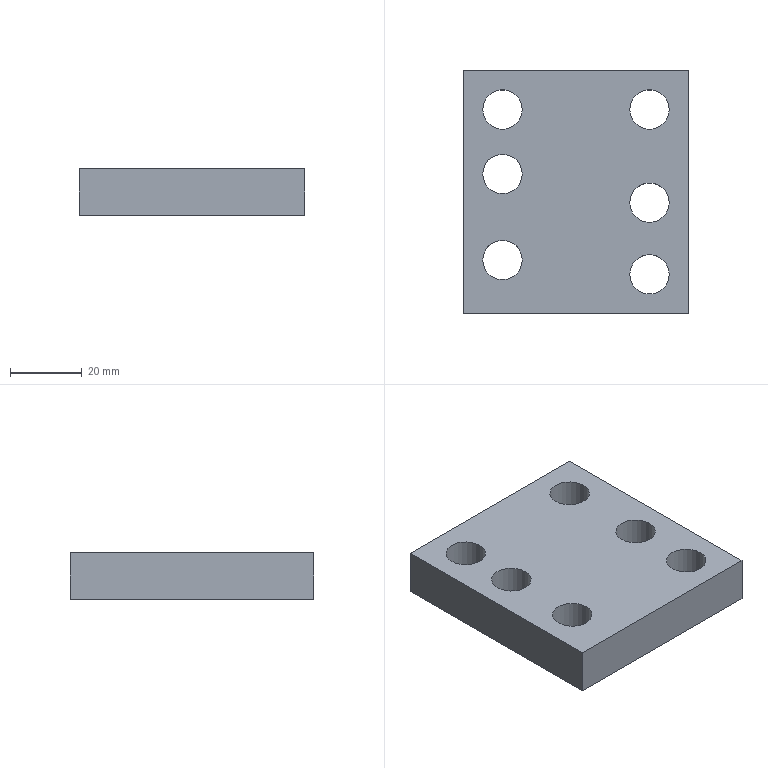Part | NX | features solid 2 | 1 solid | 12 faces | box 63 x 68 x 13 mm | volume 48279 mm3 | plane 6 | cylinder 6 | commonest cylinder face diameters 11 x6
STEP:
#1=CARTESIAN_POINT('',(1353.579,107.904,53.));
#2=VERTEX_POINT('',#1);
#3=CARTESIAN_POINT('',(1353.579,107.904,40.));
#4=VERTEX_POINT('',#3);
#5=CARTESIAN_POINT('',(1353.579,107.904,40.));
#6=DIRECTION('',(0.,0.,1.));
#7=VECTOR('',#6,1000.);
#8=LINE('',#5,#7);
#9=EDGE_CURVE('',#2,#4,#8,.F.);
#10=ORIENTED_EDGE('',*,*,#9,.T.);
#11=CARTESIAN_POINT('',(1416.579,107.904,40.));
#12=VERTEX_POINT('',#11);
#13=CARTESIAN_POINT('',(1385.079,107.904,40.));
#14=DIRECTION('',(1.,0.,0.));
#15=VECTOR('',#14,1000.);
#16=LINE('',#13,#15);
#17=EDGE_CURVE('',#12,#4,#16,.F.);
#18=ORIENTED_EDGE('',*,*,#17,.F.);
#19=CARTESIAN_POINT('',(1416.579,107.904,53.));
#20=VERTEX_POINT('',#19);
#21=CARTESIAN_POINT('',(1416.579,107.904,40.));
#22=DIRECTION('',(0.,0.,1.));
#23=VECTOR('',#22,1000.);
#24=LINE('',#21,#23);
#25=EDGE_CURVE('',#20,#12,#24,.F.);
#26=ORIENTED_EDGE('',*,*,#25,.F.);
#27=CARTESIAN_POINT('',(2186.158,107.904,53.));
#28=DIRECTION('',(1.,0.,0.));
#29=VECTOR('',#28,1000.);
#30=LINE('',#27,#29);
#31=EDGE_CURVE('',#20,#2,#30,.F.);
#32=ORIENTED_EDGE('',*,*,#31,.T.);
#33=EDGE_LOOP('',(#10,#18,#26,#32));
#34=FACE_BOUND('',#33,.T.);
#35=CARTESIAN_POINT('',(1385.079,107.904,40.));
#36=DIRECTION('',(0.,1.,0.));
#37=DIRECTION('',(1.,0.,0.));
#38=AXIS2_PLACEMENT_3D('',#35,#36,#37);
#39=PLANE('',#38);
#40=ADVANCED_FACE('',(#34),#39,.F.);
#41=ORIENTED_EDGE('',*,*,#25,.T.);
#42=CARTESIAN_POINT('',(1416.579,175.904,40.));
#43=VERTEX_POINT('',#42);
#44=CARTESIAN_POINT('',(1416.579,141.904,40.));
#45=DIRECTION('',(0.,1.,0.));
#46=VECTOR('',#45,1000.);
#47=LINE('',#44,#46);
#48=EDGE_CURVE('',#43,#12,#47,.F.);
#49=ORIENTED_EDGE('',*,*,#48,.F.);
#50=CARTESIAN_POINT('',(1416.579,175.904,53.));
#51=VERTEX_POINT('',#50);
#52=CARTESIAN_POINT('',(1416.579,175.904,40.));
#53=DIRECTION('',(0.,0.,1.));
#54=VECTOR('',#53,1000.);
#55=LINE('',#52,#54);
#56=EDGE_CURVE('',#51,#43,#55,.F.);
#57=ORIENTED_EDGE('',*,*,#56,.F.);
#58=CARTESIAN_POINT('',(1416.579,0.000000688,53.));
#59=DIRECTION('',(0.,1.,0.));
#60=VECTOR('',#59,1000.);
#61=LINE('',#58,#60);
#62=EDGE_CURVE('',#51,#20,#61,.F.);
#63=ORIENTED_EDGE('',*,*,#62,.T.);
#64=EDGE_LOOP('',(#41,#49,#57,#63));
#65=FACE_BOUND('',#64,.T.);
#66=CARTESIAN_POINT('',(1416.579,141.904,40.));
#67=DIRECTION('',(-1.,0.,0.));
#68=DIRECTION('',(0.,1.,0.));
#69=AXIS2_PLACEMENT_3D('',#66,#67,#68);
#70=PLANE('',#69);
#71=ADVANCED_FACE('',(#65),#70,.F.);
#72=ORIENTED_EDGE('',*,*,#56,.T.);
#73=CARTESIAN_POINT('',(1353.579,175.904,40.));
#74=VERTEX_POINT('',#73);
#75=CARTESIAN_POINT('',(1385.079,175.904,40.));
#76=DIRECTION('',(-1.,0.,0.));
#77=VECTOR('',#76,1000.);
#78=LINE('',#75,#77);
#79=EDGE_CURVE('',#74,#43,#78,.F.);
#80=ORIENTED_EDGE('',*,*,#79,.F.);
#81=CARTESIAN_POINT('',(1353.579,175.904,53.));
#82=VERTEX_POINT('',#81);
#83=CARTESIAN_POINT('',(1353.579,175.904,40.));
#84=DIRECTION('',(0.,0.,1.));
#85=VECTOR('',#84,1000.);
#86=LINE('',#83,#85);
#87=EDGE_CURVE('',#82,#74,#86,.F.);
#88=ORIENTED_EDGE('',*,*,#87,.F.);
#89=CARTESIAN_POINT('',(2186.158,175.904,53.));
#90=DIRECTION('',(-1.,0.,0.));
#91=VECTOR('',#90,1000.);
#92=LINE('',#89,#91);
#93=EDGE_CURVE('',#82,#51,#92,.F.);
#94=ORIENTED_EDGE('',*,*,#93,.T.);
#95=EDGE_LOOP('',(#72,#80,#88,#94));
#96=FACE_BOUND('',#95,.T.);
#97=CARTESIAN_POINT('',(1385.079,175.904,40.));
#98=DIRECTION('',(0.,-1.,0.));
#99=DIRECTION('',(-1.,0.,0.));
#100=AXIS2_PLACEMENT_3D('',#97,#98,#99);
#101=PLANE('',#100);
#102=ADVANCED_FACE('',(#96),#101,.F.);
#103=CARTESIAN_POINT('',(1370.079,146.904,40.));
#104=VERTEX_POINT('',#103);
#105=CARTESIAN_POINT('',(1364.579,146.904,40.));
#106=DIRECTION('',(0.,0.,-1.));
#107=DIRECTION('',(1.,0.,0.));
#108=AXIS2_PLACEMENT_3D('',#105,#106,#107);
#109=CIRCLE('',#108,5.5);
#110=EDGE_CURVE('',#104,#104,#109,.T.);
#111=ORIENTED_EDGE('',*,*,#110,.T.);
#112=EDGE_LOOP('',(#111));
#113=FACE_BOUND('',#112,.T.);
#114=CARTESIAN_POINT('',(1359.079,146.904,53.));
#115=VERTEX_POINT('',#114);
#116=CARTESIAN_POINT('',(1364.579,146.904,53.));
#117=DIRECTION('',(0.,0.,-1.));
#118=DIRECTION('',(-1.,0.,0.));
#119=AXIS2_PLACEMENT_3D('',#116,#117,#118);
#120=CIRCLE('',#119,5.5);
#121=EDGE_CURVE('',#115,#115,#120,.T.);
#122=ORIENTED_EDGE('',*,*,#121,.F.);
#123=EDGE_LOOP('',(#122));
#124=FACE_BOUND('',#123,.T.);
#125=CARTESIAN_POINT('',(1364.579,146.904,40.));
#126=DIRECTION('',(0.,0.,-1.));
#127=DIRECTION('',(1.,0.,0.));
#128=AXIS2_PLACEMENT_3D('',#125,#126,#127);
#129=CYLINDRICAL_SURFACE('',#128,5.5);
#130=ADVANCED_FACE('',(#113,#124),#129,.F.);
#131=CARTESIAN_POINT('',(1411.079,138.904,40.));
#132=VERTEX_POINT('',#131);
#133=CARTESIAN_POINT('',(1405.579,138.904,40.));
#134=DIRECTION('',(0.,0.,-1.));
#135=DIRECTION('',(1.,0.,0.));
#136=AXIS2_PLACEMENT_3D('',#133,#134,#135);
#137=CIRCLE('',#136,5.5);
#138=EDGE_CURVE('',#132,#132,#137,.F.);
#139=ORIENTED_EDGE('',*,*,#138,.F.);
#140=EDGE_LOOP('',(#139));
#141=FACE_BOUND('',#140,.T.);
#142=CARTESIAN_POINT('',(1400.079,138.904,53.));
#143=VERTEX_POINT('',#142);
#144=CARTESIAN_POINT('',(1405.579,138.904,53.));
#145=DIRECTION('',(0.,0.,-1.));
#146=DIRECTION('',(-1.,0.,0.));
#147=AXIS2_PLACEMENT_3D('',#144,#145,#146);
#148=CIRCLE('',#147,5.5);
#149=EDGE_CURVE('',#143,#143,#148,.F.);
#150=ORIENTED_EDGE('',*,*,#149,.T.);
#151=EDGE_LOOP('',(#150));
#152=FACE_BOUND('',#151,.T.);
#153=CARTESIAN_POINT('',(1405.579,138.904,40.));
#154=DIRECTION('',(0.,0.,-1.));
#155=DIRECTION('',(1.,0.,0.));
#156=AXIS2_PLACEMENT_3D('',#153,#154,#155);
#157=CYLINDRICAL_SURFACE('',#156,5.5);
#158=ADVANCED_FACE('',(#141,#152),#157,.F.);
#159=CARTESIAN_POINT('',(1370.079,122.904,40.));
#160=VERTEX_POINT('',#159);
#161=CARTESIAN_POINT('',(1364.579,122.904,40.));
#162=DIRECTION('',(0.,0.,-1.));
#163=DIRECTION('',(1.,0.,0.));
#164=AXIS2_PLACEMENT_3D('',#161,#162,#163);
#165=CIRCLE('',#164,5.5);
#166=EDGE_CURVE('',#160,#160,#165,.T.);
#167=ORIENTED_EDGE('',*,*,#166,.T.);
#168=EDGE_LOOP('',(#167));
#169=FACE_BOUND('',#168,.T.);
#170=CARTESIAN_POINT('',(1359.079,122.904,53.));
#171=VERTEX_POINT('',#170);
#172=CARTESIAN_POINT('',(1364.579,122.904,53.));
#173=DIRECTION('',(0.,0.,-1.));
#174=DIRECTION('',(-1.,0.,0.));
#175=AXIS2_PLACEMENT_3D('',#172,#173,#174);
#176=CIRCLE('',#175,5.5);
#177=EDGE_CURVE('',#171,#171,#176,.T.);
#178=ORIENTED_EDGE('',*,*,#177,.F.);
#179=EDGE_LOOP('',(#178));
#180=FACE_BOUND('',#179,.T.);
#181=CARTESIAN_POINT('',(1364.579,122.904,40.));
#182=DIRECTION('',(0.,0.,-1.));
#183=DIRECTION('',(1.,0.,0.));
#184=AXIS2_PLACEMENT_3D('',#181,#182,#183);
#185=CYLINDRICAL_SURFACE('',#184,5.5);
#186=ADVANCED_FACE('',(#169,#180),#185,.F.);
#187=CARTESIAN_POINT('',(1370.079,164.904,40.));
#188=VERTEX_POINT('',#187);
#189=CARTESIAN_POINT('',(1364.579,164.904,40.));
#190=DIRECTION('',(0.,0.,-1.));
#191=DIRECTION('',(1.,0.,0.));
#192=AXIS2_PLACEMENT_3D('',#189,#190,#191);
#193=CIRCLE('',#192,5.5);
#194=EDGE_CURVE('',#188,#188,#193,.T.);
#195=ORIENTED_EDGE('',*,*,#194,.T.);
#196=EDGE_LOOP('',(#195));
#197=FACE_BOUND('',#196,.T.);
#198=CARTESIAN_POINT('',(1359.079,164.904,53.));
#199=VERTEX_POINT('',#198);
#200=CARTESIAN_POINT('',(1364.579,164.904,53.));
#201=DIRECTION('',(0.,0.,-1.));
#202=DIRECTION('',(-1.,0.,0.));
#203=AXIS2_PLACEMENT_3D('',#200,#201,#202);
#204=CIRCLE('',#203,5.5);
#205=EDGE_CURVE('',#199,#199,#204,.T.);
#206=ORIENTED_EDGE('',*,*,#205,.F.);
#207=EDGE_LOOP('',(#206));
#208=FACE_BOUND('',#207,.T.);
#209=CARTESIAN_POINT('',(1364.579,164.904,40.));
#210=DIRECTION('',(0.,0.,-1.));
#211=DIRECTION('',(1.,0.,0.));
#212=AXIS2_PLACEMENT_3D('',#209,#210,#211);
#213=CYLINDRICAL_SURFACE('',#212,5.5);
#214=ADVANCED_FACE('',(#197,#208),#213,.F.);
#215=CARTESIAN_POINT('',(1411.079,164.904,40.));
#216=VERTEX_POINT('',#215);
#217=CARTESIAN_POINT('',(1405.579,164.904,40.));
#218=DIRECTION('',(0.,0.,-1.));
#219=DIRECTION('',(1.,0.,0.));
#220=AXIS2_PLACEMENT_3D('',#217,#218,#219);
#221=CIRCLE('',#220,5.5);
#222=EDGE_CURVE('',#216,#216,#221,.T.);
#223=ORIENTED_EDGE('',*,*,#222,.T.);
#224=EDGE_LOOP('',(#223));
#225=FACE_BOUND('',#224,.T.);
#226=CARTESIAN_POINT('',(1400.079,164.904,53.));
#227=VERTEX_POINT('',#226);
#228=CARTESIAN_POINT('',(1405.579,164.904,53.));
#229=DIRECTION('',(0.,0.,-1.));
#230=DIRECTION('',(-1.,0.,0.));
#231=AXIS2_PLACEMENT_3D('',#228,#229,#230);
#232=CIRCLE('',#231,5.5);
#233=EDGE_CURVE('',#227,#227,#232,.T.);
#234=ORIENTED_EDGE('',*,*,#233,.F.);
#235=EDGE_LOOP('',(#234));
#236=FACE_BOUND('',#235,.T.);
#237=CARTESIAN_POINT('',(1405.579,164.904,40.));
#238=DIRECTION('',(0.,0.,-1.));
#239=DIRECTION('',(1.,0.,0.));
#240=AXIS2_PLACEMENT_3D('',#237,#238,#239);
#241=CYLINDRICAL_SURFACE('',#240,5.5);
#242=ADVANCED_FACE('',(#225,#236),#241,.F.);
#243=CARTESIAN_POINT('',(1411.079,118.904,40.));
#244=VERTEX_POINT('',#243);
#245=CARTESIAN_POINT('',(1405.579,118.904,40.));
#246=DIRECTION('',(0.,0.,-1.));
#247=DIRECTION('',(1.,0.,0.));
#248=AXIS2_PLACEMENT_3D('',#245,#246,#247);
#249=CIRCLE('',#248,5.5);
#250=EDGE_CURVE('',#244,#244,#249,.F.);
#251=ORIENTED_EDGE('',*,*,#250,.F.);
#252=EDGE_LOOP('',(#251));
#253=FACE_BOUND('',#252,.T.);
#254=CARTESIAN_POINT('',(1400.079,118.904,53.));
#255=VERTEX_POINT('',#254);
#256=CARTESIAN_POINT('',(1405.579,118.904,53.));
#257=DIRECTION('',(0.,0.,-1.));
#258=DIRECTION('',(-1.,0.,0.));
#259=AXIS2_PLACEMENT_3D('',#256,#257,#258);
#260=CIRCLE('',#259,5.5);
#261=EDGE_CURVE('',#255,#255,#260,.F.);
#262=ORIENTED_EDGE('',*,*,#261,.T.);
#263=EDGE_LOOP('',(#262));
#264=FACE_BOUND('',#263,.T.);
#265=CARTESIAN_POINT('',(1405.579,118.904,40.));
#266=DIRECTION('',(0.,0.,-1.));
#267=DIRECTION('',(1.,0.,0.));
#268=AXIS2_PLACEMENT_3D('',#265,#266,#267);
#269=CYLINDRICAL_SURFACE('',#268,5.5);
#270=ADVANCED_FACE('',(#253,#264),#269,.F.);
#271=CARTESIAN_POINT('',(1353.579,0.000000688,53.));
#272=DIRECTION('',(0.,-1.,0.));
#273=VECTOR('',#272,1000.);
#274=LINE('',#271,#273);
#275=EDGE_CURVE('',#2,#82,#274,.F.);
#276=ORIENTED_EDGE('',*,*,#275,.T.);
#277=ORIENTED_EDGE('',*,*,#87,.T.);
#278=CARTESIAN_POINT('',(1353.579,141.904,40.));
#279=DIRECTION('',(0.,-1.,0.));
#280=VECTOR('',#279,1000.);
#281=LINE('',#278,#280);
#282=EDGE_CURVE('',#4,#74,#281,.F.);
#283=ORIENTED_EDGE('',*,*,#282,.F.);
#284=ORIENTED_EDGE('',*,*,#9,.F.);
#285=EDGE_LOOP('',(#276,#277,#283,#284));
#286=FACE_BOUND('',#285,.T.);
#287=CARTESIAN_POINT('',(1353.579,141.904,40.));
#288=DIRECTION('',(1.,0.,0.));
#289=DIRECTION('',(0.,-1.,0.));
#290=AXIS2_PLACEMENT_3D('',#287,#288,#289);
#291=PLANE('',#290);
#292=ADVANCED_FACE('',(#286),#291,.F.);
#293=ORIENTED_EDGE('',*,*,#110,.F.);
#294=EDGE_LOOP('',(#293));
#295=FACE_BOUND('',#294,.T.);
#296=ORIENTED_EDGE('',*,*,#138,.T.);
#297=EDGE_LOOP('',(#296));
#298=FACE_BOUND('',#297,.T.);
#299=ORIENTED_EDGE('',*,*,#166,.F.);
#300=EDGE_LOOP('',(#299));
#301=FACE_BOUND('',#300,.T.);
#302=ORIENTED_EDGE('',*,*,#194,.F.);
#303=EDGE_LOOP('',(#302));
#304=FACE_BOUND('',#303,.T.);
#305=ORIENTED_EDGE('',*,*,#222,.F.);
#306=EDGE_LOOP('',(#305));
#307=FACE_BOUND('',#306,.T.);
#308=ORIENTED_EDGE('',*,*,#250,.T.);
#309=EDGE_LOOP('',(#308));
#310=FACE_BOUND('',#309,.T.);
#311=ORIENTED_EDGE('',*,*,#79,.T.);
#312=ORIENTED_EDGE('',*,*,#48,.T.);
#313=ORIENTED_EDGE('',*,*,#17,.T.);
#314=ORIENTED_EDGE('',*,*,#282,.T.);
#315=EDGE_LOOP('',(#311,#312,#313,#314));
#316=FACE_BOUND('',#315,.T.);
#317=CARTESIAN_POINT('',(2186.158,0.000000688,40.));
#318=DIRECTION('',(0.,0.,-1.));
#319=DIRECTION('',(1.,0.,0.));
#320=AXIS2_PLACEMENT_3D('',#317,#318,#319);
#321=PLANE('',#320);
#322=ADVANCED_FACE('',(#295,#298,#301,#304,#307,#310,#316),#321,.T.);
#323=ORIENTED_EDGE('',*,*,#121,.T.);
#324=EDGE_LOOP('',(#323));
#325=FACE_BOUND('',#324,.T.);
#326=ORIENTED_EDGE('',*,*,#149,.F.);
#327=EDGE_LOOP('',(#326));
#328=FACE_BOUND('',#327,.T.);
#329=ORIENTED_EDGE('',*,*,#177,.T.);
#330=EDGE_LOOP('',(#329));
#331=FACE_BOUND('',#330,.T.);
#332=ORIENTED_EDGE('',*,*,#205,.T.);
#333=EDGE_LOOP('',(#332));
#334=FACE_BOUND('',#333,.T.);
#335=ORIENTED_EDGE('',*,*,#233,.T.);
#336=EDGE_LOOP('',(#335));
#337=FACE_BOUND('',#336,.T.);
#338=ORIENTED_EDGE('',*,*,#261,.F.);
#339=EDGE_LOOP('',(#338));
#340=FACE_BOUND('',#339,.T.);
#341=ORIENTED_EDGE('',*,*,#93,.F.);
#342=ORIENTED_EDGE('',*,*,#275,.F.);
#343=ORIENTED_EDGE('',*,*,#31,.F.);
#344=ORIENTED_EDGE('',*,*,#62,.F.);
#345=EDGE_LOOP('',(#341,#342,#343,#344));
#346=FACE_BOUND('',#345,.T.);
#347=CARTESIAN_POINT('',(2186.158,0.000000688,53.));
#348=DIRECTION('',(0.,0.,-1.));
#349=DIRECTION('',(1.,0.,0.));
#350=AXIS2_PLACEMENT_3D('',#347,#348,#349);
#351=PLANE('',#350);
#352=ADVANCED_FACE('',(#325,#328,#331,#334,#337,#340,#346),#351,.F.);
#353=CLOSED_SHELL('',(#40,#71,#102,#130,#158,#186,#214,#242,#270,#292,#322,#352));
#354=MANIFOLD_SOLID_BREP('',#353);
#355=(LENGTH_UNIT()NAMED_UNIT(*)SI_UNIT(.MILLI.,.METRE.));
#356=UNCERTAINTY_MEASURE_WITH_UNIT(LENGTH_MEASURE(0.00001),#355,'','');
#357=(NAMED_UNIT(*)PLANE_ANGLE_UNIT()SI_UNIT($,.RADIAN.));
#358=(NAMED_UNIT(*)SI_UNIT($,.STERADIAN.)SOLID_ANGLE_UNIT());
#359=(GEOMETRIC_REPRESENTATION_CONTEXT(3)GLOBAL_UNCERTAINTY_ASSIGNED_CONTEXT((#356))GLOBAL_UNIT_ASSIGNED_CONTEXT((#355,#357,#358))REPRESENTATION_CONTEXT('',''));
#360=ADVANCED_BREP_SHAPE_REPRESENTATION('',(#354),#359);